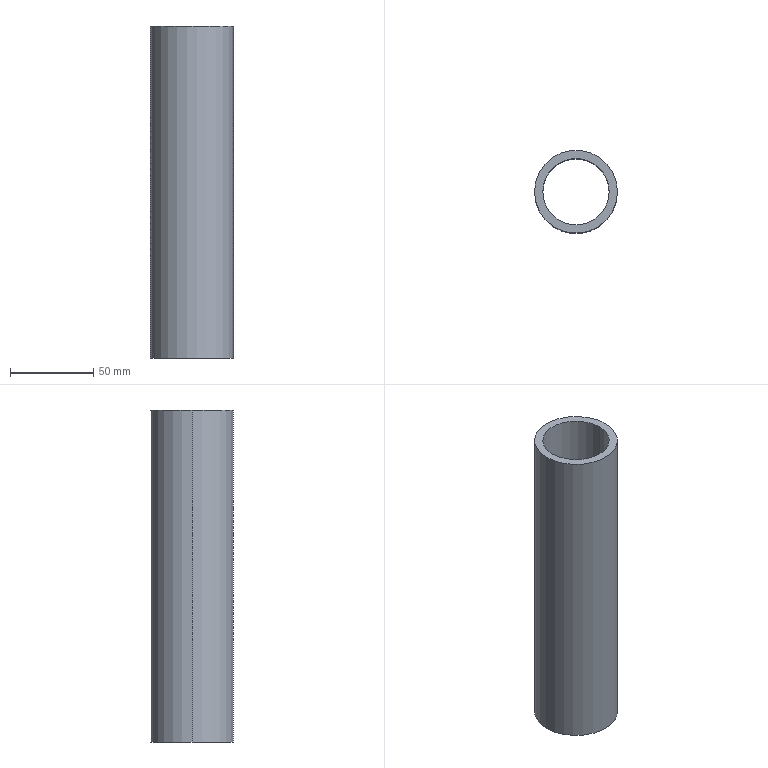Part | SolidWorks | features Extrusion 1 | 1 solid | 6 faces | box 50 x 50 x 200 mm | volume 141372 mm3 | cylinder 4 | plane 2 | commonest cylinder face diameters 40 x2 50 x2
STEP:
#1=CARTESIAN_POINT('',(-20.,0.,200.));
#2=VERTEX_POINT('',#1);
#3=CARTESIAN_POINT('',(20.,0.,200.));
#4=VERTEX_POINT('',#3);
#5=CARTESIAN_POINT('',(0.,0.,200.));
#6=DIRECTION('',(0.,0.,1.));
#7=DIRECTION('',(1.,0.,0.));
#8=AXIS2_PLACEMENT_3D('',#5,#6,#7);
#9=CIRCLE('',#8,20.);
#10=EDGE_CURVE('',#2,#4,#9,.T.);
#11=ORIENTED_EDGE('',*,*,#10,.T.);
#12=CARTESIAN_POINT('',(20.,0.,0.));
#13=VERTEX_POINT('',#12);
#14=CARTESIAN_POINT('',(20.,0.,200.));
#15=DIRECTION('',(0.,0.,-1.));
#16=VECTOR('',#15,1000.);
#17=LINE('',#14,#16);
#18=EDGE_CURVE('',#4,#13,#17,.T.);
#19=ORIENTED_EDGE('',*,*,#18,.T.);
#20=CARTESIAN_POINT('',(-20.,0.,0.));
#21=VERTEX_POINT('',#20);
#22=CARTESIAN_POINT('',(0.,0.,0.));
#23=DIRECTION('',(0.,0.,1.));
#24=DIRECTION('',(1.,0.,0.));
#25=AXIS2_PLACEMENT_3D('',#22,#23,#24);
#26=CIRCLE('',#25,20.);
#27=EDGE_CURVE('',#21,#13,#26,.T.);
#28=ORIENTED_EDGE('',*,*,#27,.F.);
#29=CARTESIAN_POINT('',(-20.,0.,200.));
#30=DIRECTION('',(0.,0.,-1.));
#31=VECTOR('',#30,1000.);
#32=LINE('',#29,#31);
#33=EDGE_CURVE('',#2,#21,#32,.T.);
#34=ORIENTED_EDGE('',*,*,#33,.F.);
#35=EDGE_LOOP('',(#11,#19,#28,#34));
#36=FACE_OUTER_BOUND('',#35,.T.);
#37=CARTESIAN_POINT('',(0.,0.,200.));
#38=DIRECTION('',(0.,0.,-1.));
#39=DIRECTION('',(-1.,0.,0.));
#40=AXIS2_PLACEMENT_3D('',#37,#38,#39);
#41=CYLINDRICAL_SURFACE('',#40,20.);
#42=ADVANCED_FACE('',(#36),#41,.F.);
#43=CARTESIAN_POINT('',(25.,0.,200.));
#44=VERTEX_POINT('',#43);
#45=CARTESIAN_POINT('',(-25.,0.,200.));
#46=VERTEX_POINT('',#45);
#47=CARTESIAN_POINT('',(0.,0.,200.));
#48=DIRECTION('',(0.,0.,1.));
#49=DIRECTION('',(1.,0.,0.));
#50=AXIS2_PLACEMENT_3D('',#47,#48,#49);
#51=CIRCLE('',#50,25.);
#52=EDGE_CURVE('',#44,#46,#51,.T.);
#53=ORIENTED_EDGE('',*,*,#52,.F.);
#54=CARTESIAN_POINT('',(25.,0.,0.));
#55=VERTEX_POINT('',#54);
#56=CARTESIAN_POINT('',(25.,0.,200.));
#57=DIRECTION('',(0.,0.,-1.));
#58=VECTOR('',#57,1000.);
#59=LINE('',#56,#58);
#60=EDGE_CURVE('',#44,#55,#59,.T.);
#61=ORIENTED_EDGE('',*,*,#60,.T.);
#62=CARTESIAN_POINT('',(-25.,0.,0.));
#63=VERTEX_POINT('',#62);
#64=CARTESIAN_POINT('',(0.,0.,0.));
#65=DIRECTION('',(0.,0.,1.));
#66=DIRECTION('',(1.,0.,0.));
#67=AXIS2_PLACEMENT_3D('',#64,#65,#66);
#68=CIRCLE('',#67,25.);
#69=EDGE_CURVE('',#55,#63,#68,.T.);
#70=ORIENTED_EDGE('',*,*,#69,.T.);
#71=CARTESIAN_POINT('',(-25.,0.,200.));
#72=DIRECTION('',(0.,0.,-1.));
#73=VECTOR('',#72,1000.);
#74=LINE('',#71,#73);
#75=EDGE_CURVE('',#46,#63,#74,.T.);
#76=ORIENTED_EDGE('',*,*,#75,.F.);
#77=EDGE_LOOP('',(#53,#61,#70,#76));
#78=FACE_OUTER_BOUND('',#77,.T.);
#79=CARTESIAN_POINT('',(0.,0.,200.));
#80=DIRECTION('',(0.,0.,-1.));
#81=DIRECTION('',(-1.,0.,0.));
#82=AXIS2_PLACEMENT_3D('',#79,#80,#81);
#83=CYLINDRICAL_SURFACE('',#82,25.);
#84=ADVANCED_FACE('',(#78),#83,.T.);
#85=CARTESIAN_POINT('',(0.,0.,200.));
#86=DIRECTION('',(0.,0.,1.));
#87=DIRECTION('',(1.,0.,0.));
#88=AXIS2_PLACEMENT_3D('',#85,#86,#87);
#89=CIRCLE('',#88,25.);
#90=EDGE_CURVE('',#46,#44,#89,.T.);
#91=ORIENTED_EDGE('',*,*,#90,.T.);
#92=ORIENTED_EDGE('',*,*,#52,.T.);
#93=EDGE_LOOP('',(#91,#92));
#94=FACE_OUTER_BOUND('',#93,.T.);
#95=ORIENTED_EDGE('',*,*,#10,.F.);
#96=CARTESIAN_POINT('',(0.,0.,200.));
#97=DIRECTION('',(0.,0.,1.));
#98=DIRECTION('',(1.,0.,0.));
#99=AXIS2_PLACEMENT_3D('',#96,#97,#98);
#100=CIRCLE('',#99,20.);
#101=EDGE_CURVE('',#4,#2,#100,.T.);
#102=ORIENTED_EDGE('',*,*,#101,.F.);
#103=EDGE_LOOP('',(#95,#102));
#104=FACE_BOUND('',#103,.T.);
#105=CARTESIAN_POINT('',(0.,0.,200.));
#106=DIRECTION('',(0.,0.,1.));
#107=DIRECTION('',(1.,0.,0.));
#108=AXIS2_PLACEMENT_3D('',#105,#106,#107);
#109=PLANE('',#108);
#110=ADVANCED_FACE('',(#94,#104),#109,.T.);
#111=CARTESIAN_POINT('',(0.,0.,0.));
#112=DIRECTION('',(0.,0.,1.));
#113=DIRECTION('',(1.,0.,0.));
#114=AXIS2_PLACEMENT_3D('',#111,#112,#113);
#115=CIRCLE('',#114,25.);
#116=EDGE_CURVE('',#63,#55,#115,.T.);
#117=ORIENTED_EDGE('',*,*,#116,.F.);
#118=ORIENTED_EDGE('',*,*,#69,.F.);
#119=EDGE_LOOP('',(#117,#118));
#120=FACE_OUTER_BOUND('',#119,.T.);
#121=ORIENTED_EDGE('',*,*,#27,.T.);
#122=CARTESIAN_POINT('',(0.,0.,0.));
#123=DIRECTION('',(0.,0.,1.));
#124=DIRECTION('',(1.,0.,0.));
#125=AXIS2_PLACEMENT_3D('',#122,#123,#124);
#126=CIRCLE('',#125,20.);
#127=EDGE_CURVE('',#13,#21,#126,.T.);
#128=ORIENTED_EDGE('',*,*,#127,.T.);
#129=EDGE_LOOP('',(#121,#128));
#130=FACE_BOUND('',#129,.T.);
#131=CARTESIAN_POINT('',(0.,0.,0.));
#132=DIRECTION('',(0.,0.,1.));
#133=DIRECTION('',(1.,0.,0.));
#134=AXIS2_PLACEMENT_3D('',#131,#132,#133);
#135=PLANE('',#134);
#136=ADVANCED_FACE('',(#120,#130),#135,.F.);
#137=ORIENTED_EDGE('',*,*,#60,.F.);
#138=ORIENTED_EDGE('',*,*,#90,.F.);
#139=ORIENTED_EDGE('',*,*,#75,.T.);
#140=ORIENTED_EDGE('',*,*,#116,.T.);
#141=EDGE_LOOP('',(#137,#138,#139,#140));
#142=FACE_OUTER_BOUND('',#141,.T.);
#143=CARTESIAN_POINT('',(0.,0.,200.));
#144=DIRECTION('',(0.,0.,-1.));
#145=DIRECTION('',(-1.,0.,0.));
#146=AXIS2_PLACEMENT_3D('',#143,#144,#145);
#147=CYLINDRICAL_SURFACE('',#146,25.);
#148=ADVANCED_FACE('',(#142),#147,.T.);
#149=ORIENTED_EDGE('',*,*,#18,.F.);
#150=ORIENTED_EDGE('',*,*,#101,.T.);
#151=ORIENTED_EDGE('',*,*,#33,.T.);
#152=ORIENTED_EDGE('',*,*,#127,.F.);
#153=EDGE_LOOP('',(#149,#150,#151,#152));
#154=FACE_OUTER_BOUND('',#153,.T.);
#155=CARTESIAN_POINT('',(0.,0.,200.));
#156=DIRECTION('',(0.,0.,-1.));
#157=DIRECTION('',(-1.,0.,0.));
#158=AXIS2_PLACEMENT_3D('',#155,#156,#157);
#159=CYLINDRICAL_SURFACE('',#158,20.);
#160=ADVANCED_FACE('',(#154),#159,.F.);
#161=CLOSED_SHELL('',(#42,#84,#110,#136,#148,#160));
#162=MANIFOLD_SOLID_BREP('',#161);
#163=CARTESIAN_POINT('',(0.,0.,0.));
#164=DIRECTION('',(0.,0.,1.));
#165=DIRECTION('',(1.,0.,0.));
#166=AXIS2_PLACEMENT_3D('',#163,#164,#165);
#167=(LENGTH_UNIT()NAMED_UNIT(*)SI_UNIT(.MILLI.,.METRE.));
#168=UNCERTAINTY_MEASURE_WITH_UNIT(LENGTH_MEASURE(0.00001),#167,'','');
#169=(NAMED_UNIT(*)PLANE_ANGLE_UNIT()SI_UNIT($,.RADIAN.));
#170=(NAMED_UNIT(*)SI_UNIT($,.STERADIAN.)SOLID_ANGLE_UNIT());
#171=(GEOMETRIC_REPRESENTATION_CONTEXT(3)GLOBAL_UNCERTAINTY_ASSIGNED_CONTEXT((#168))GLOBAL_UNIT_ASSIGNED_CONTEXT((#167,#169,#170))REPRESENTATION_CONTEXT('',''));
#172=ADVANCED_BREP_SHAPE_REPRESENTATION('',(#162,#166),#171);